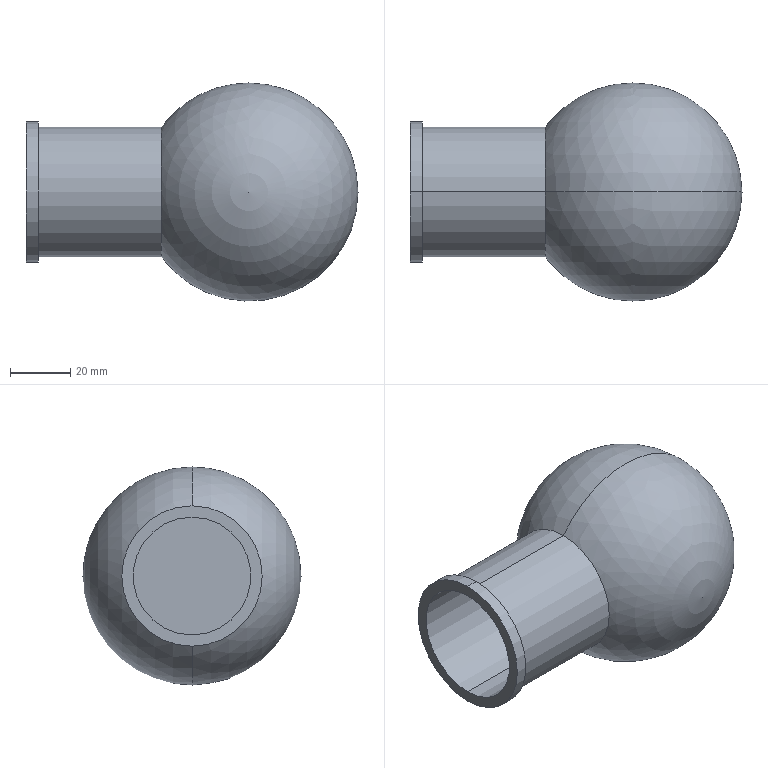Part | SolidWorks | features BaseBody 1, Revolution 1 | 1 solid | 11 faces | box 109.98 x 72.246 x 72.246 mm | volume 221727 mm3 | cylinder 6 | plane 3 | sphere 2 | commonest cylinder face diameters 39 x2 43 x2 46.5 x2
STEP:
#1=CARTESIAN_POINT('',(130.94,0.,0.));
#2=VERTEX_POINT('',#1);
#3=CARTESIAN_POINT('',(65.789,0.,21.5));
#4=VERTEX_POINT('',#3);
#5=CARTESIAN_POINT('',(94.817,0.,0.));
#6=DIRECTION('',(0.,-1.,0.));
#7=DIRECTION('',(0.,0.,-1.));
#8=AXIS2_PLACEMENT_3D('',#5,#6,#7);
#9=CIRCLE('',#8,36.123);
#10=EDGE_CURVE('',#2,#4,#9,.T.);
#11=ORIENTED_EDGE('',*,*,#10,.F.);
#12=CARTESIAN_POINT('',(65.789,0.,-21.5));
#13=VERTEX_POINT('',#12);
#14=CARTESIAN_POINT('',(94.817,0.,0.));
#15=DIRECTION('',(0.,1.,0.));
#16=DIRECTION('',(0.,0.,1.));
#17=AXIS2_PLACEMENT_3D('',#14,#15,#16);
#18=CIRCLE('',#17,36.123);
#19=EDGE_CURVE('',#2,#13,#18,.T.);
#20=ORIENTED_EDGE('',*,*,#19,.T.);
#21=CARTESIAN_POINT('',(65.789,0.,0.));
#22=DIRECTION('',(-1.,0.,0.));
#23=DIRECTION('',(0.,0.,1.));
#24=AXIS2_PLACEMENT_3D('',#21,#22,#23);
#25=CIRCLE('',#24,21.5);
#26=EDGE_CURVE('',#4,#13,#25,.T.);
#27=ORIENTED_EDGE('',*,*,#26,.F.);
#28=EDGE_LOOP('',(#11,#20,#27));
#29=FACE_OUTER_BOUND('',#28,.T.);
#30=CARTESIAN_POINT('',(94.817,0.,0.));
#31=DIRECTION('',(0.,1.,0.));
#32=DIRECTION('',(0.,0.,1.));
#33=AXIS2_PLACEMENT_3D('',#30,#31,#32);
#34=SPHERICAL_SURFACE('',#33,36.123);
#35=ADVANCED_FACE('',(#29),#34,.T.);
#36=CARTESIAN_POINT('',(24.96,0.,23.25));
#37=VERTEX_POINT('',#36);
#38=CARTESIAN_POINT('',(24.96,0.,-23.25));
#39=VERTEX_POINT('',#38);
#40=CARTESIAN_POINT('',(24.96,0.,0.));
#41=DIRECTION('',(-1.,0.,0.));
#42=DIRECTION('',(0.,0.,1.));
#43=AXIS2_PLACEMENT_3D('',#40,#41,#42);
#44=CIRCLE('',#43,23.25);
#45=EDGE_CURVE('',#37,#39,#44,.T.);
#46=ORIENTED_EDGE('',*,*,#45,.T.);
#47=CARTESIAN_POINT('',(20.96,0.,-23.25));
#48=VERTEX_POINT('',#47);
#49=CARTESIAN_POINT('',(0.,0.,-23.25));
#50=DIRECTION('',(-1.,0.,0.));
#51=VECTOR('',#50,1000.);
#52=LINE('',#49,#51);
#53=EDGE_CURVE('',#39,#48,#52,.T.);
#54=ORIENTED_EDGE('',*,*,#53,.T.);
#55=CARTESIAN_POINT('',(20.96,0.,23.25));
#56=VERTEX_POINT('',#55);
#57=CARTESIAN_POINT('',(20.96,0.,0.));
#58=DIRECTION('',(1.,0.,0.));
#59=DIRECTION('',(0.,0.,1.));
#60=AXIS2_PLACEMENT_3D('',#57,#58,#59);
#61=CIRCLE('',#60,23.25);
#62=EDGE_CURVE('',#48,#56,#61,.T.);
#63=ORIENTED_EDGE('',*,*,#62,.T.);
#64=CARTESIAN_POINT('',(0.,0.,23.25));
#65=DIRECTION('',(-1.,0.,0.));
#66=VECTOR('',#65,1000.);
#67=LINE('',#64,#66);
#68=EDGE_CURVE('',#37,#56,#67,.T.);
#69=ORIENTED_EDGE('',*,*,#68,.F.);
#70=EDGE_LOOP('',(#46,#54,#63,#69));
#71=FACE_OUTER_BOUND('',#70,.T.);
#72=CARTESIAN_POINT('',(0.,0.,0.));
#73=DIRECTION('',(-1.,0.,0.));
#74=DIRECTION('',(0.,0.,1.));
#75=AXIS2_PLACEMENT_3D('',#72,#73,#74);
#76=CYLINDRICAL_SURFACE('',#75,23.25);
#77=ADVANCED_FACE('',(#71),#76,.T.);
#78=ORIENTED_EDGE('',*,*,#26,.T.);
#79=CARTESIAN_POINT('',(24.96,0.,-21.5));
#80=VERTEX_POINT('',#79);
#81=CARTESIAN_POINT('',(0.,0.,-21.5));
#82=DIRECTION('',(-1.,0.,0.));
#83=VECTOR('',#82,1000.);
#84=LINE('',#81,#83);
#85=EDGE_CURVE('',#13,#80,#84,.T.);
#86=ORIENTED_EDGE('',*,*,#85,.T.);
#87=CARTESIAN_POINT('',(24.96,0.,21.5));
#88=VERTEX_POINT('',#87);
#89=CARTESIAN_POINT('',(24.96,0.,0.));
#90=DIRECTION('',(1.,0.,0.));
#91=DIRECTION('',(0.,0.,1.));
#92=AXIS2_PLACEMENT_3D('',#89,#90,#91);
#93=CIRCLE('',#92,21.5);
#94=EDGE_CURVE('',#80,#88,#93,.T.);
#95=ORIENTED_EDGE('',*,*,#94,.T.);
#96=CARTESIAN_POINT('',(0.,0.,21.5));
#97=DIRECTION('',(-1.,0.,0.));
#98=VECTOR('',#97,1000.);
#99=LINE('',#96,#98);
#100=EDGE_CURVE('',#4,#88,#99,.T.);
#101=ORIENTED_EDGE('',*,*,#100,.F.);
#102=EDGE_LOOP('',(#78,#86,#95,#101));
#103=FACE_OUTER_BOUND('',#102,.T.);
#104=CARTESIAN_POINT('',(0.,0.,0.));
#105=DIRECTION('',(-1.,0.,0.));
#106=DIRECTION('',(0.,0.,1.));
#107=AXIS2_PLACEMENT_3D('',#104,#105,#106);
#108=CYLINDRICAL_SURFACE('',#107,21.5);
#109=ADVANCED_FACE('',(#103),#108,.T.);
#110=CARTESIAN_POINT('',(51.484,0.,-19.5));
#111=VERTEX_POINT('',#110);
#112=CARTESIAN_POINT('',(51.484,0.,19.5));
#113=VERTEX_POINT('',#112);
#114=CARTESIAN_POINT('',(51.484,0.,0.));
#115=DIRECTION('',(-1.,0.,0.));
#116=DIRECTION('',(0.,0.,-1.));
#117=AXIS2_PLACEMENT_3D('',#114,#115,#116);
#118=CIRCLE('',#117,19.5);
#119=EDGE_CURVE('',#111,#113,#118,.T.);
#120=ORIENTED_EDGE('',*,*,#119,.F.);
#121=CARTESIAN_POINT('',(20.96,0.,-19.5));
#122=VERTEX_POINT('',#121);
#123=CARTESIAN_POINT('',(0.,0.,-19.5));
#124=DIRECTION('',(-1.,0.,0.));
#125=VECTOR('',#124,1000.);
#126=LINE('',#123,#125);
#127=EDGE_CURVE('',#111,#122,#126,.T.);
#128=ORIENTED_EDGE('',*,*,#127,.T.);
#129=CARTESIAN_POINT('',(20.96,0.,19.5));
#130=VERTEX_POINT('',#129);
#131=CARTESIAN_POINT('',(20.96,0.,0.));
#132=DIRECTION('',(1.,0.,0.));
#133=DIRECTION('',(0.,0.,1.));
#134=AXIS2_PLACEMENT_3D('',#131,#132,#133);
#135=CIRCLE('',#134,19.5);
#136=EDGE_CURVE('',#130,#122,#135,.T.);
#137=ORIENTED_EDGE('',*,*,#136,.F.);
#138=CARTESIAN_POINT('',(0.,0.,19.5));
#139=DIRECTION('',(-1.,0.,0.));
#140=VECTOR('',#139,1000.);
#141=LINE('',#138,#140);
#142=EDGE_CURVE('',#113,#130,#141,.T.);
#143=ORIENTED_EDGE('',*,*,#142,.F.);
#144=EDGE_LOOP('',(#120,#128,#137,#143));
#145=FACE_OUTER_BOUND('',#144,.T.);
#146=CARTESIAN_POINT('',(0.,0.,0.));
#147=DIRECTION('',(-1.,0.,0.));
#148=DIRECTION('',(0.,0.,1.));
#149=AXIS2_PLACEMENT_3D('',#146,#147,#148);
#150=CYLINDRICAL_SURFACE('',#149,19.5);
#151=ADVANCED_FACE('',(#145),#150,.F.);
#152=ORIENTED_EDGE('',*,*,#127,.F.);
#153=CARTESIAN_POINT('',(51.484,0.,0.));
#154=DIRECTION('',(-1.,0.,0.));
#155=DIRECTION('',(0.,0.,-1.));
#156=AXIS2_PLACEMENT_3D('',#153,#154,#155);
#157=CIRCLE('',#156,19.5);
#158=EDGE_CURVE('',#113,#111,#157,.T.);
#159=ORIENTED_EDGE('',*,*,#158,.F.);
#160=ORIENTED_EDGE('',*,*,#142,.T.);
#161=CARTESIAN_POINT('',(20.96,0.,0.));
#162=DIRECTION('',(1.,0.,0.));
#163=DIRECTION('',(0.,0.,1.));
#164=AXIS2_PLACEMENT_3D('',#161,#162,#163);
#165=CIRCLE('',#164,19.5);
#166=EDGE_CURVE('',#122,#130,#165,.T.);
#167=ORIENTED_EDGE('',*,*,#166,.F.);
#168=EDGE_LOOP('',(#152,#159,#160,#167));
#169=FACE_OUTER_BOUND('',#168,.T.);
#170=CARTESIAN_POINT('',(0.,0.,0.));
#171=DIRECTION('',(-1.,0.,0.));
#172=DIRECTION('',(0.,0.,1.));
#173=AXIS2_PLACEMENT_3D('',#170,#171,#172);
#174=CYLINDRICAL_SURFACE('',#173,19.5);
#175=ADVANCED_FACE('',(#169),#174,.F.);
#176=ORIENTED_EDGE('',*,*,#136,.T.);
#177=ORIENTED_EDGE('',*,*,#166,.T.);
#178=EDGE_LOOP('',(#176,#177));
#179=FACE_BOUND('',#178,.T.);
#180=CARTESIAN_POINT('',(20.96,0.,0.));
#181=DIRECTION('',(1.,0.,0.));
#182=DIRECTION('',(0.,0.,1.));
#183=AXIS2_PLACEMENT_3D('',#180,#181,#182);
#184=CIRCLE('',#183,23.25);
#185=EDGE_CURVE('',#56,#48,#184,.T.);
#186=ORIENTED_EDGE('',*,*,#185,.F.);
#187=ORIENTED_EDGE('',*,*,#62,.F.);
#188=EDGE_LOOP('',(#186,#187));
#189=FACE_OUTER_BOUND('',#188,.T.);
#190=CARTESIAN_POINT('',(20.96,0.,0.));
#191=DIRECTION('',(1.,0.,0.));
#192=DIRECTION('',(0.,0.,-1.));
#193=AXIS2_PLACEMENT_3D('',#190,#191,#192);
#194=PLANE('',#193);
#195=ADVANCED_FACE('',(#179,#189),#194,.F.);
#196=ORIENTED_EDGE('',*,*,#53,.F.);
#197=CARTESIAN_POINT('',(24.96,0.,0.));
#198=DIRECTION('',(-1.,0.,0.));
#199=DIRECTION('',(0.,0.,1.));
#200=AXIS2_PLACEMENT_3D('',#197,#198,#199);
#201=CIRCLE('',#200,23.25);
#202=EDGE_CURVE('',#39,#37,#201,.T.);
#203=ORIENTED_EDGE('',*,*,#202,.T.);
#204=ORIENTED_EDGE('',*,*,#68,.T.);
#205=ORIENTED_EDGE('',*,*,#185,.T.);
#206=EDGE_LOOP('',(#196,#203,#204,#205));
#207=FACE_OUTER_BOUND('',#206,.T.);
#208=CARTESIAN_POINT('',(0.,0.,0.));
#209=DIRECTION('',(-1.,0.,0.));
#210=DIRECTION('',(0.,0.,1.));
#211=AXIS2_PLACEMENT_3D('',#208,#209,#210);
#212=CYLINDRICAL_SURFACE('',#211,23.25);
#213=ADVANCED_FACE('',(#207),#212,.T.);
#214=ORIENTED_EDGE('',*,*,#85,.F.);
#215=CARTESIAN_POINT('',(65.789,0.,0.));
#216=DIRECTION('',(-1.,0.,0.));
#217=DIRECTION('',(0.,0.,1.));
#218=AXIS2_PLACEMENT_3D('',#215,#216,#217);
#219=CIRCLE('',#218,21.5);
#220=EDGE_CURVE('',#13,#4,#219,.T.);
#221=ORIENTED_EDGE('',*,*,#220,.T.);
#222=ORIENTED_EDGE('',*,*,#100,.T.);
#223=CARTESIAN_POINT('',(24.96,0.,0.));
#224=DIRECTION('',(1.,0.,0.));
#225=DIRECTION('',(0.,0.,1.));
#226=AXIS2_PLACEMENT_3D('',#223,#224,#225);
#227=CIRCLE('',#226,21.5);
#228=EDGE_CURVE('',#88,#80,#227,.T.);
#229=ORIENTED_EDGE('',*,*,#228,.T.);
#230=EDGE_LOOP('',(#214,#221,#222,#229));
#231=FACE_OUTER_BOUND('',#230,.T.);
#232=CARTESIAN_POINT('',(0.,0.,0.));
#233=DIRECTION('',(-1.,0.,0.));
#234=DIRECTION('',(0.,0.,1.));
#235=AXIS2_PLACEMENT_3D('',#232,#233,#234);
#236=CYLINDRICAL_SURFACE('',#235,21.5);
#237=ADVANCED_FACE('',(#231),#236,.T.);
#238=ORIENTED_EDGE('',*,*,#228,.F.);
#239=ORIENTED_EDGE('',*,*,#94,.F.);
#240=EDGE_LOOP('',(#238,#239));
#241=FACE_BOUND('',#240,.T.);
#242=ORIENTED_EDGE('',*,*,#45,.F.);
#243=ORIENTED_EDGE('',*,*,#202,.F.);
#244=EDGE_LOOP('',(#242,#243));
#245=FACE_OUTER_BOUND('',#244,.T.);
#246=CARTESIAN_POINT('',(24.96,0.,0.));
#247=DIRECTION('',(-1.,0.,0.));
#248=DIRECTION('',(0.,0.,1.));
#249=AXIS2_PLACEMENT_3D('',#246,#247,#248);
#250=PLANE('',#249);
#251=ADVANCED_FACE('',(#241,#245),#250,.F.);
#252=ORIENTED_EDGE('',*,*,#158,.T.);
#253=ORIENTED_EDGE('',*,*,#119,.T.);
#254=EDGE_LOOP('',(#252,#253));
#255=FACE_OUTER_BOUND('',#254,.T.);
#256=CARTESIAN_POINT('',(51.484,0.,0.));
#257=DIRECTION('',(1.,0.,0.));
#258=DIRECTION('',(0.,0.,-1.));
#259=AXIS2_PLACEMENT_3D('',#256,#257,#258);
#260=PLANE('',#259);
#261=ADVANCED_FACE('',(#255),#260,.F.);
#262=ORIENTED_EDGE('',*,*,#19,.F.);
#263=ORIENTED_EDGE('',*,*,#10,.T.);
#264=ORIENTED_EDGE('',*,*,#220,.F.);
#265=EDGE_LOOP('',(#262,#263,#264));
#266=FACE_OUTER_BOUND('',#265,.T.);
#267=CARTESIAN_POINT('',(94.817,0.,0.));
#268=DIRECTION('',(0.,1.,0.));
#269=DIRECTION('',(0.,0.,1.));
#270=AXIS2_PLACEMENT_3D('',#267,#268,#269);
#271=SPHERICAL_SURFACE('',#270,36.123);
#272=ADVANCED_FACE('',(#266),#271,.T.);
#273=CLOSED_SHELL('',(#35,#77,#109,#151,#175,#195,#213,#237,#251,#261,#272));
#274=MANIFOLD_SOLID_BREP('',#273);
#275=CARTESIAN_POINT('',(0.,0.,0.));
#276=DIRECTION('',(0.,0.,1.));
#277=DIRECTION('',(1.,0.,0.));
#278=AXIS2_PLACEMENT_3D('',#275,#276,#277);
#279=(LENGTH_UNIT()NAMED_UNIT(*)SI_UNIT(.MILLI.,.METRE.));
#280=UNCERTAINTY_MEASURE_WITH_UNIT(LENGTH_MEASURE(0.00001),#279,'','');
#281=(NAMED_UNIT(*)PLANE_ANGLE_UNIT()SI_UNIT($,.RADIAN.));
#282=(NAMED_UNIT(*)SI_UNIT($,.STERADIAN.)SOLID_ANGLE_UNIT());
#283=(GEOMETRIC_REPRESENTATION_CONTEXT(3)GLOBAL_UNCERTAINTY_ASSIGNED_CONTEXT((#280))GLOBAL_UNIT_ASSIGNED_CONTEXT((#279,#281,#282))REPRESENTATION_CONTEXT('',''));
#284=ADVANCED_BREP_SHAPE_REPRESENTATION('',(#274,#278),#283);